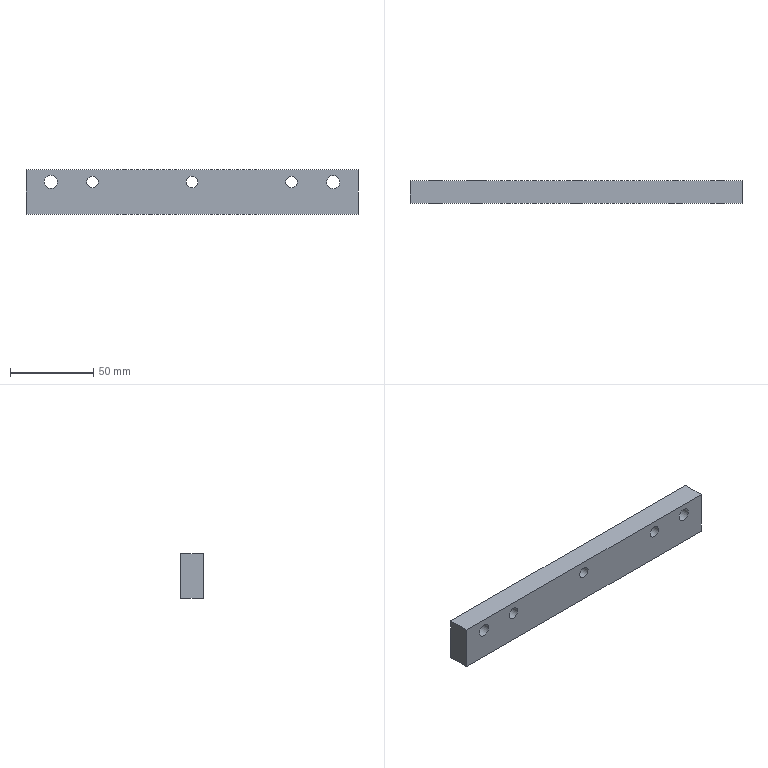Part | STEP file | SN10_002_006_GUIA | 1 solid | 17 faces | box 200 x 13.5 x 27 mm | volume 68797 mm3 | plane 9 | cylinder 8 | commonest cylinder face diameters 7 x3 11 x3 8 x2
STEP:
#1=CARTESIAN_POINT('',(0.,0.,0.));
#2=DIRECTION('',(0.,0.,1.));
#3=DIRECTION('',(1.,0.,0.));
#4=AXIS2_PLACEMENT_3D('',#1,#2,#3);
#5=CARTESIAN_POINT('',(88.51,228.5,59.418));
#6=VERTEX_POINT('',#5);
#7=CARTESIAN_POINT('',(85.,228.5,57.5));
#8=DIRECTION('',(0.,-1.,0.));
#9=DIRECTION('',(1.,0.,0.));
#10=AXIS2_PLACEMENT_3D('',#7,#8,#9);
#11=CIRCLE('',#10,4.);
#12=CARTESIAN_POINT('',(85.,228.4,57.5));
#13=DIRECTION('',(0.,-1.,0.));
#14=DIRECTION('',(0.8776,0.,0.4794));
#15=AXIS2_PLACEMENT_3D('',#12,#13,#14);
#16=CYLINDRICAL_SURFACE('',#15,4.);
#17=CARTESIAN_POINT('',(-0.5,-0.1));
#18=DIRECTION('',(1.,0.));
#19=VECTOR('',#18,1.);
#20=LINE('',#17,#19);
#21=(GEOMETRIC_REPRESENTATION_CONTEXT(2)PARAMETRIC_REPRESENTATION_CONTEXT()REPRESENTATION_CONTEXT('',''));
#22=DEFINITIONAL_REPRESENTATION('',(#20),#21);
#23=PCURVE('',#16,#22);
#24=CARTESIAN_POINT('',(0.,228.5,65.));
#25=DIRECTION('',(0.,-1.,0.));
#26=DIRECTION('',(0.,0.,-1.));
#27=AXIS2_PLACEMENT_3D('',#24,#25,#26);
#28=PLANE('',#27);
#29=CARTESIAN_POINT('',(7.5,85.));
#30=DIRECTION('',(0.,1.));
#31=AXIS2_PLACEMENT_2D('',#29,#30);
#32=CIRCLE('',#31,4.);
#33=(GEOMETRIC_REPRESENTATION_CONTEXT(2)PARAMETRIC_REPRESENTATION_CONTEXT()REPRESENTATION_CONTEXT('',''));
#34=DEFINITIONAL_REPRESENTATION('',(#32),#33);
#35=PCURVE('',#28,#34);
#36=SURFACE_CURVE('',#11,(#23,#35),.PCURVE_S1.);
#37=EDGE_CURVE('',#6,#6,#36,.T.);
#38=ORIENTED_EDGE('',*,*,#37,.T.);
#39=CARTESIAN_POINT('',(88.51,215.,59.418));
#40=VERTEX_POINT('',#39);
#41=CARTESIAN_POINT('',(88.51,228.5,59.418));
#42=CARTESIAN_POINT('',(88.51,215.,59.418));
#43=B_SPLINE_CURVE_WITH_KNOTS('',1,(#41,#42),.UNSPECIFIED.,.F.,.F.,(2,2),(-0.1,13.4),.PIECEWISE_BEZIER_KNOTS.);
#44=CARTESIAN_POINT('',(6.283,0.));
#45=DIRECTION('',(0.,1.));
#46=VECTOR('',#45,1.);
#47=LINE('',#44,#46);
#48=(GEOMETRIC_REPRESENTATION_CONTEXT(2)PARAMETRIC_REPRESENTATION_CONTEXT()REPRESENTATION_CONTEXT('',''));
#49=DEFINITIONAL_REPRESENTATION('',(#47),#48);
#50=PCURVE('',#16,#49);
#51=CARTESIAN_POINT('',(0.,0.));
#52=DIRECTION('',(0.,1.));
#53=VECTOR('',#52,1.);
#54=LINE('',#51,#53);
#55=(GEOMETRIC_REPRESENTATION_CONTEXT(2)PARAMETRIC_REPRESENTATION_CONTEXT()REPRESENTATION_CONTEXT('',''));
#56=DEFINITIONAL_REPRESENTATION('',(#54),#55);
#57=PCURVE('',#16,#56);
#58=SEAM_CURVE('',#43,(#50,#57),.PCURVE_S1.);
#59=EDGE_CURVE('',#6,#40,#58,.T.);
#60=ORIENTED_EDGE('',*,*,#59,.T.);
#61=CARTESIAN_POINT('',(85.,215.,57.5));
#62=DIRECTION('',(0.,-1.,0.));
#63=DIRECTION('',(1.,0.,0.));
#64=AXIS2_PLACEMENT_3D('',#61,#62,#63);
#65=CIRCLE('',#64,4.);
#66=CARTESIAN_POINT('',(-0.5,13.4));
#67=DIRECTION('',(1.,0.));
#68=VECTOR('',#67,1.);
#69=LINE('',#66,#68);
#70=(GEOMETRIC_REPRESENTATION_CONTEXT(2)PARAMETRIC_REPRESENTATION_CONTEXT()REPRESENTATION_CONTEXT('',''));
#71=DEFINITIONAL_REPRESENTATION('',(#69),#70);
#72=PCURVE('',#16,#71);
#73=CARTESIAN_POINT('',(0.,215.,38.));
#74=DIRECTION('',(0.,1.,0.));
#75=DIRECTION('',(0.,0.,1.));
#76=AXIS2_PLACEMENT_3D('',#73,#74,#75);
#77=PLANE('',#76);
#78=CARTESIAN_POINT('',(19.5,89.));
#79=CARTESIAN_POINT('',(26.428,89.));
#80=CARTESIAN_POINT('',(22.964,83.));
#81=CARTESIAN_POINT('',(19.5,77.));
#82=CARTESIAN_POINT('',(16.036,83.));
#83=CARTESIAN_POINT('',(12.572,89.));
#84=CARTESIAN_POINT('',(19.5,89.));
#85=(BOUNDED_CURVE()B_SPLINE_CURVE(2,(#78,#79,#80,#81,#82,#83,#84),.UNSPECIFIED.,.T.,.F.)B_SPLINE_CURVE_WITH_KNOTS((1,2,2,2,2,1),(-2.094,0.,2.094,4.189,6.283,8.378),.UNSPECIFIED.)CURVE()GEOMETRIC_REPRESENTATION_ITEM()RATIONAL_B_SPLINE_CURVE((1.,0.5,1.,0.5,1.,0.5,1.))REPRESENTATION_ITEM(''));
#86=(GEOMETRIC_REPRESENTATION_CONTEXT(2)PARAMETRIC_REPRESENTATION_CONTEXT()REPRESENTATION_CONTEXT('',''));
#87=DEFINITIONAL_REPRESENTATION('',(#85),#86);
#88=PCURVE('',#77,#87);
#89=SURFACE_CURVE('',#65,(#72,#88),.PCURVE_S1.);
#90=EDGE_CURVE('',#40,#40,#89,.T.);
#91=ORIENTED_EDGE('',*,*,#90,.F.);
#92=ORIENTED_EDGE('',*,*,#59,.F.);
#93=EDGE_LOOP('',(#38,#60,#91,#92));
#94=FACE_BOUND('',#93,.F.);
#95=ADVANCED_FACE('',(#94),#16,.F.);
#96=CARTESIAN_POINT('',(-100.,228.5,65.));
#97=VERTEX_POINT('',#96);
#98=CARTESIAN_POINT('',(100.,228.5,65.));
#99=VERTEX_POINT('',#98);
#100=CARTESIAN_POINT('',(-100.,228.5,65.));
#101=DIRECTION('',(1.,0.,0.));
#102=VECTOR('',#101,1.);
#103=LINE('',#100,#102);
#104=CARTESIAN_POINT('',(0.,215.,65.));
#105=DIRECTION('',(0.,0.,-1.));
#106=DIRECTION('',(-1.,0.,0.));
#107=AXIS2_PLACEMENT_3D('',#104,#105,#106);
#108=PLANE('',#107);
#109=CARTESIAN_POINT('',(100.,13.5));
#110=DIRECTION('',(-1.,0.));
#111=VECTOR('',#110,1.);
#112=LINE('',#109,#111);
#113=(GEOMETRIC_REPRESENTATION_CONTEXT(2)PARAMETRIC_REPRESENTATION_CONTEXT()REPRESENTATION_CONTEXT('',''));
#114=DEFINITIONAL_REPRESENTATION('',(#112),#113);
#115=PCURVE('',#108,#114);
#116=CARTESIAN_POINT('',(0.,-100.));
#117=DIRECTION('',(0.,1.));
#118=VECTOR('',#117,1.);
#119=LINE('',#116,#118);
#120=(GEOMETRIC_REPRESENTATION_CONTEXT(2)PARAMETRIC_REPRESENTATION_CONTEXT()REPRESENTATION_CONTEXT('',''));
#121=DEFINITIONAL_REPRESENTATION('',(#119),#120);
#122=PCURVE('',#28,#121);
#123=SURFACE_CURVE('',#103,(#115,#122),.PCURVE_S1.);
#124=EDGE_CURVE('',#97,#99,#123,.T.);
#125=ORIENTED_EDGE('',*,*,#124,.F.);
#126=CARTESIAN_POINT('',(-100.,215.,65.));
#127=VERTEX_POINT('',#126);
#128=CARTESIAN_POINT('',(-100.,215.,65.));
#129=DIRECTION('',(0.,1.,0.));
#130=VECTOR('',#129,1.);
#131=LINE('',#128,#130);
#132=CARTESIAN_POINT('',(100.,0.));
#133=DIRECTION('',(0.,1.));
#134=VECTOR('',#133,1.);
#135=LINE('',#132,#134);
#136=(GEOMETRIC_REPRESENTATION_CONTEXT(2)PARAMETRIC_REPRESENTATION_CONTEXT()REPRESENTATION_CONTEXT('',''));
#137=DEFINITIONAL_REPRESENTATION('',(#135),#136);
#138=PCURVE('',#108,#137);
#139=CARTESIAN_POINT('',(-100.,0.,0.));
#140=DIRECTION('',(1.,0.,0.));
#141=DIRECTION('',(0.,0.,-1.));
#142=AXIS2_PLACEMENT_3D('',#139,#140,#141);
#143=PLANE('',#142);
#144=CARTESIAN_POINT('',(-65.,215.));
#145=DIRECTION('',(0.,1.));
#146=VECTOR('',#145,1.);
#147=LINE('',#144,#146);
#148=(GEOMETRIC_REPRESENTATION_CONTEXT(2)PARAMETRIC_REPRESENTATION_CONTEXT()REPRESENTATION_CONTEXT('',''));
#149=DEFINITIONAL_REPRESENTATION('',(#147),#148);
#150=PCURVE('',#143,#149);
#151=SURFACE_CURVE('',#131,(#138,#150),.PCURVE_S1.);
#152=EDGE_CURVE('',#127,#97,#151,.T.);
#153=ORIENTED_EDGE('',*,*,#152,.F.);
#154=CARTESIAN_POINT('',(100.,215.,65.));
#155=VERTEX_POINT('',#154);
#156=CARTESIAN_POINT('',(-100.,215.,65.));
#157=DIRECTION('',(1.,0.,0.));
#158=VECTOR('',#157,1.);
#159=LINE('',#156,#158);
#160=CARTESIAN_POINT('',(100.,0.));
#161=DIRECTION('',(-1.,0.));
#162=VECTOR('',#161,1.);
#163=LINE('',#160,#162);
#164=(GEOMETRIC_REPRESENTATION_CONTEXT(2)PARAMETRIC_REPRESENTATION_CONTEXT()REPRESENTATION_CONTEXT('',''));
#165=DEFINITIONAL_REPRESENTATION('',(#163),#164);
#166=PCURVE('',#108,#165);
#167=CARTESIAN_POINT('',(27.,-100.));
#168=DIRECTION('',(0.,1.));
#169=VECTOR('',#168,1.);
#170=LINE('',#167,#169);
#171=(GEOMETRIC_REPRESENTATION_CONTEXT(2)PARAMETRIC_REPRESENTATION_CONTEXT()REPRESENTATION_CONTEXT('',''));
#172=DEFINITIONAL_REPRESENTATION('',(#170),#171);
#173=PCURVE('',#77,#172);
#174=SURFACE_CURVE('',#159,(#166,#173),.PCURVE_S1.);
#175=EDGE_CURVE('',#127,#155,#174,.T.);
#176=ORIENTED_EDGE('',*,*,#175,.T.);
#177=CARTESIAN_POINT('',(100.,215.,65.));
#178=DIRECTION('',(0.,1.,0.));
#179=VECTOR('',#178,1.);
#180=LINE('',#177,#179);
#181=CARTESIAN_POINT('',(-100.,0.));
#182=DIRECTION('',(0.,1.));
#183=VECTOR('',#182,1.);
#184=LINE('',#181,#183);
#185=(GEOMETRIC_REPRESENTATION_CONTEXT(2)PARAMETRIC_REPRESENTATION_CONTEXT()REPRESENTATION_CONTEXT('',''));
#186=DEFINITIONAL_REPRESENTATION('',(#184),#185);
#187=PCURVE('',#108,#186);
#188=CARTESIAN_POINT('',(100.,0.,0.));
#189=DIRECTION('',(1.,0.,0.));
#190=DIRECTION('',(0.,0.,-1.));
#191=AXIS2_PLACEMENT_3D('',#188,#189,#190);
#192=PLANE('',#191);
#193=CARTESIAN_POINT('',(-65.,215.));
#194=DIRECTION('',(0.,1.));
#195=VECTOR('',#194,1.);
#196=LINE('',#193,#195);
#197=(GEOMETRIC_REPRESENTATION_CONTEXT(2)PARAMETRIC_REPRESENTATION_CONTEXT()REPRESENTATION_CONTEXT('',''));
#198=DEFINITIONAL_REPRESENTATION('',(#196),#197);
#199=PCURVE('',#192,#198);
#200=SURFACE_CURVE('',#180,(#187,#199),.PCURVE_S1.);
#201=EDGE_CURVE('',#155,#99,#200,.T.);
#202=ORIENTED_EDGE('',*,*,#201,.T.);
#203=EDGE_LOOP('',(#125,#153,#176,#202));
#204=FACE_BOUND('',#203,.T.);
#205=ADVANCED_FACE('',(#204),#108,.F.);
#206=CARTESIAN_POINT('',(-100.,228.5,38.));
#207=VERTEX_POINT('',#206);
#208=CARTESIAN_POINT('',(-100.,228.5,65.));
#209=DIRECTION('',(0.,0.,-1.));
#210=VECTOR('',#209,1.);
#211=LINE('',#208,#210);
#212=CARTESIAN_POINT('',(-65.,228.5));
#213=DIRECTION('',(1.,0.));
#214=VECTOR('',#213,1.);
#215=LINE('',#212,#214);
#216=(GEOMETRIC_REPRESENTATION_CONTEXT(2)PARAMETRIC_REPRESENTATION_CONTEXT()REPRESENTATION_CONTEXT('',''));
#217=DEFINITIONAL_REPRESENTATION('',(#215),#216);
#218=PCURVE('',#143,#217);
#219=CARTESIAN_POINT('',(0.,-100.));
#220=DIRECTION('',(1.,0.));
#221=VECTOR('',#220,1.);
#222=LINE('',#219,#221);
#223=(GEOMETRIC_REPRESENTATION_CONTEXT(2)PARAMETRIC_REPRESENTATION_CONTEXT()REPRESENTATION_CONTEXT('',''));
#224=DEFINITIONAL_REPRESENTATION('',(#222),#223);
#225=PCURVE('',#28,#224);
#226=SURFACE_CURVE('',#211,(#218,#225),.PCURVE_S1.);
#227=EDGE_CURVE('',#97,#207,#226,.T.);
#228=ORIENTED_EDGE('',*,*,#227,.T.);
#229=CARTESIAN_POINT('',(-100.,215.,38.));
#230=VERTEX_POINT('',#229);
#231=CARTESIAN_POINT('',(-100.,228.5,38.));
#232=DIRECTION('',(0.,-1.,0.));
#233=VECTOR('',#232,1.);
#234=LINE('',#231,#233);
#235=CARTESIAN_POINT('',(-38.,228.5));
#236=DIRECTION('',(0.,-1.));
#237=VECTOR('',#236,1.);
#238=LINE('',#235,#237);
#239=(GEOMETRIC_REPRESENTATION_CONTEXT(2)PARAMETRIC_REPRESENTATION_CONTEXT()REPRESENTATION_CONTEXT('',''));
#240=DEFINITIONAL_REPRESENTATION('',(#238),#239);
#241=PCURVE('',#143,#240);
#242=CARTESIAN_POINT('',(0.,228.5,38.));
#243=DIRECTION('',(0.,0.,1.));
#244=DIRECTION('',(1.,0.,0.));
#245=AXIS2_PLACEMENT_3D('',#242,#243,#244);
#246=PLANE('',#245);
#247=CARTESIAN_POINT('',(-100.,0.));
#248=DIRECTION('',(0.,-1.));
#249=VECTOR('',#248,1.);
#250=LINE('',#247,#249);
#251=(GEOMETRIC_REPRESENTATION_CONTEXT(2)PARAMETRIC_REPRESENTATION_CONTEXT()REPRESENTATION_CONTEXT('',''));
#252=DEFINITIONAL_REPRESENTATION('',(#250),#251);
#253=PCURVE('',#246,#252);
#254=SURFACE_CURVE('',#234,(#241,#253),.PCURVE_S1.);
#255=EDGE_CURVE('',#207,#230,#254,.T.);
#256=ORIENTED_EDGE('',*,*,#255,.T.);
#257=CARTESIAN_POINT('',(-100.,215.,38.));
#258=DIRECTION('',(0.,0.,1.));
#259=VECTOR('',#258,1.);
#260=LINE('',#257,#259);
#261=CARTESIAN_POINT('',(-38.,215.));
#262=DIRECTION('',(-1.,0.));
#263=VECTOR('',#262,1.);
#264=LINE('',#261,#263);
#265=(GEOMETRIC_REPRESENTATION_CONTEXT(2)PARAMETRIC_REPRESENTATION_CONTEXT()REPRESENTATION_CONTEXT('',''));
#266=DEFINITIONAL_REPRESENTATION('',(#264),#265);
#267=PCURVE('',#143,#266);
#268=CARTESIAN_POINT('',(0.,-100.));
#269=DIRECTION('',(1.,0.));
#270=VECTOR('',#269,1.);
#271=LINE('',#268,#270);
#272=(GEOMETRIC_REPRESENTATION_CONTEXT(2)PARAMETRIC_REPRESENTATION_CONTEXT()REPRESENTATION_CONTEXT('',''));
#273=DEFINITIONAL_REPRESENTATION('',(#271),#272);
#274=PCURVE('',#77,#273);
#275=SURFACE_CURVE('',#260,(#267,#274),.PCURVE_S1.);
#276=EDGE_CURVE('',#230,#127,#275,.T.);
#277=ORIENTED_EDGE('',*,*,#276,.T.);
#278=ORIENTED_EDGE('',*,*,#152,.T.);
#279=EDGE_LOOP('',(#228,#256,#277,#278));
#280=FACE_BOUND('',#279,.T.);
#281=ADVANCED_FACE('',(#280),#143,.F.);
#282=CARTESIAN_POINT('',(55.173,228.5,54.863));
#283=VERTEX_POINT('',#282);
#284=CARTESIAN_POINT('',(60.,228.5,57.5));
#285=DIRECTION('',(0.,-1.,0.));
#286=DIRECTION('',(1.,0.,0.));
#287=AXIS2_PLACEMENT_3D('',#284,#285,#286);
#288=CIRCLE('',#287,5.5);
#289=CARTESIAN_POINT('',(60.,228.4,57.5));
#290=DIRECTION('',(0.,-1.,0.));
#291=DIRECTION('',(0.8776,0.,0.4794));
#292=AXIS2_PLACEMENT_3D('',#289,#290,#291);
#293=CYLINDRICAL_SURFACE('',#292,5.5);
#294=CARTESIAN_POINT('',(-0.5,-0.1));
#295=DIRECTION('',(1.,0.));
#296=VECTOR('',#295,1.);
#297=LINE('',#294,#296);
#298=(GEOMETRIC_REPRESENTATION_CONTEXT(2)PARAMETRIC_REPRESENTATION_CONTEXT()REPRESENTATION_CONTEXT('',''));
#299=DEFINITIONAL_REPRESENTATION('',(#297),#298);
#300=PCURVE('',#293,#299);
#301=CARTESIAN_POINT('',(7.5,60.));
#302=DIRECTION('',(0.,1.));
#303=AXIS2_PLACEMENT_2D('',#301,#302);
#304=CIRCLE('',#303,5.5);
#305=(GEOMETRIC_REPRESENTATION_CONTEXT(2)PARAMETRIC_REPRESENTATION_CONTEXT()REPRESENTATION_CONTEXT('',''));
#306=DEFINITIONAL_REPRESENTATION('',(#304),#305);
#307=PCURVE('',#28,#306);
#308=SURFACE_CURVE('',#288,(#300,#307),.PCURVE_S1.);
#309=EDGE_CURVE('',#283,#283,#308,.T.);
#310=ORIENTED_EDGE('',*,*,#309,.T.);
#311=CARTESIAN_POINT('',(55.173,221.5,54.863));
#312=VERTEX_POINT('',#311);
#313=CARTESIAN_POINT('',(55.173,228.5,54.863));
#314=CARTESIAN_POINT('',(55.173,221.5,54.863));
#315=B_SPLINE_CURVE_WITH_KNOTS('',1,(#313,#314),.UNSPECIFIED.,.F.,.F.,(2,2),(-0.1,6.9),.PIECEWISE_BEZIER_KNOTS.);
#316=CARTESIAN_POINT('',(9.425,0.));
#317=DIRECTION('',(0.,1.));
#318=VECTOR('',#317,1.);
#319=LINE('',#316,#318);
#320=(GEOMETRIC_REPRESENTATION_CONTEXT(2)PARAMETRIC_REPRESENTATION_CONTEXT()REPRESENTATION_CONTEXT('',''));
#321=DEFINITIONAL_REPRESENTATION('',(#319),#320);
#322=PCURVE('',#293,#321);
#323=CARTESIAN_POINT('',(3.142,0.));
#324=DIRECTION('',(0.,1.));
#325=VECTOR('',#324,1.);
#326=LINE('',#323,#325);
#327=(GEOMETRIC_REPRESENTATION_CONTEXT(2)PARAMETRIC_REPRESENTATION_CONTEXT()REPRESENTATION_CONTEXT('',''));
#328=DEFINITIONAL_REPRESENTATION('',(#326),#327);
#329=PCURVE('',#293,#328);
#330=SEAM_CURVE('',#315,(#322,#329),.PCURVE_S1.);
#331=EDGE_CURVE('',#283,#312,#330,.T.);
#332=ORIENTED_EDGE('',*,*,#331,.T.);
#333=CARTESIAN_POINT('',(60.,221.5,57.5));
#334=DIRECTION('',(0.,-1.,0.));
#335=DIRECTION('',(1.,0.,0.));
#336=AXIS2_PLACEMENT_3D('',#333,#334,#335);
#337=CIRCLE('',#336,5.5);
#338=CARTESIAN_POINT('',(-0.5,6.9));
#339=DIRECTION('',(1.,0.));
#340=VECTOR('',#339,1.);
#341=LINE('',#338,#340);
#342=(GEOMETRIC_REPRESENTATION_CONTEXT(2)PARAMETRIC_REPRESENTATION_CONTEXT()REPRESENTATION_CONTEXT('',''));
#343=DEFINITIONAL_REPRESENTATION('',(#341),#342);
#344=PCURVE('',#293,#343);
#345=CARTESIAN_POINT('',(63.5,221.5,57.5));
#346=DIRECTION('',(0.,-1.,0.));
#347=DIRECTION('',(0.,0.,-1.));
#348=AXIS2_PLACEMENT_3D('',#345,#346,#347);
#349=PLANE('',#348);
#350=CARTESIAN_POINT('',(0.,-3.5));
#351=DIRECTION('',(0.,1.));
#352=AXIS2_PLACEMENT_2D('',#350,#351);
#353=CIRCLE('',#352,5.5);
#354=(GEOMETRIC_REPRESENTATION_CONTEXT(2)PARAMETRIC_REPRESENTATION_CONTEXT()REPRESENTATION_CONTEXT('',''));
#355=DEFINITIONAL_REPRESENTATION('',(#353),#354);
#356=PCURVE('',#349,#355);
#357=SURFACE_CURVE('',#337,(#344,#356),.PCURVE_S1.);
#358=EDGE_CURVE('',#312,#312,#357,.T.);
#359=ORIENTED_EDGE('',*,*,#358,.F.);
#360=ORIENTED_EDGE('',*,*,#331,.F.);
#361=EDGE_LOOP('',(#310,#332,#359,#360));
#362=FACE_BOUND('',#361,.F.);
#363=ADVANCED_FACE('',(#362),#293,.F.);
#364=CARTESIAN_POINT('',(-4.827,228.5,54.863));
#365=VERTEX_POINT('',#364);
#366=CARTESIAN_POINT('',(0.,228.5,57.5));
#367=DIRECTION('',(0.,-1.,0.));
#368=DIRECTION('',(1.,0.,0.));
#369=AXIS2_PLACEMENT_3D('',#366,#367,#368);
#370=CIRCLE('',#369,5.5);
#371=CARTESIAN_POINT('',(0.,228.4,57.5));
#372=DIRECTION('',(0.,-1.,0.));
#373=DIRECTION('',(0.8776,0.,0.4794));
#374=AXIS2_PLACEMENT_3D('',#371,#372,#373);
#375=CYLINDRICAL_SURFACE('',#374,5.5);
#376=CARTESIAN_POINT('',(-0.5,-0.1));
#377=DIRECTION('',(1.,0.));
#378=VECTOR('',#377,1.);
#379=LINE('',#376,#378);
#380=(GEOMETRIC_REPRESENTATION_CONTEXT(2)PARAMETRIC_REPRESENTATION_CONTEXT()REPRESENTATION_CONTEXT('',''));
#381=DEFINITIONAL_REPRESENTATION('',(#379),#380);
#382=PCURVE('',#375,#381);
#383=CARTESIAN_POINT('',(7.5,0.));
#384=DIRECTION('',(0.,1.));
#385=AXIS2_PLACEMENT_2D('',#383,#384);
#386=CIRCLE('',#385,5.5);
#387=(GEOMETRIC_REPRESENTATION_CONTEXT(2)PARAMETRIC_REPRESENTATION_CONTEXT()REPRESENTATION_CONTEXT('',''));
#388=DEFINITIONAL_REPRESENTATION('',(#386),#387);
#389=PCURVE('',#28,#388);
#390=SURFACE_CURVE('',#370,(#382,#389),.PCURVE_S1.);
#391=EDGE_CURVE('',#365,#365,#390,.T.);
#392=ORIENTED_EDGE('',*,*,#391,.T.);
#393=CARTESIAN_POINT('',(-4.827,221.5,54.863));
#394=VERTEX_POINT('',#393);
#395=CARTESIAN_POINT('',(-4.827,228.5,54.863));
#396=CARTESIAN_POINT('',(-4.827,221.5,54.863));
#397=B_SPLINE_CURVE_WITH_KNOTS('',1,(#395,#396),.UNSPECIFIED.,.F.,.F.,(2,2),(-0.1,6.9),.PIECEWISE_BEZIER_KNOTS.);
#398=CARTESIAN_POINT('',(9.425,0.));
#399=DIRECTION('',(0.,1.));
#400=VECTOR('',#399,1.);
#401=LINE('',#398,#400);
#402=(GEOMETRIC_REPRESENTATION_CONTEXT(2)PARAMETRIC_REPRESENTATION_CONTEXT()REPRESENTATION_CONTEXT('',''));
#403=DEFINITIONAL_REPRESENTATION('',(#401),#402);
#404=PCURVE('',#375,#403);
#405=CARTESIAN_POINT('',(3.142,0.));
#406=DIRECTION('',(0.,1.));
#407=VECTOR('',#406,1.);
#408=LINE('',#405,#407);
#409=(GEOMETRIC_REPRESENTATION_CONTEXT(2)PARAMETRIC_REPRESENTATION_CONTEXT()REPRESENTATION_CONTEXT('',''));
#410=DEFINITIONAL_REPRESENTATION('',(#408),#409);
#411=PCURVE('',#375,#410);
#412=SEAM_CURVE('',#397,(#404,#411),.PCURVE_S1.);
#413=EDGE_CURVE('',#365,#394,#412,.T.);
#414=ORIENTED_EDGE('',*,*,#413,.T.);
#415=CARTESIAN_POINT('',(0.,221.5,57.5));
#416=DIRECTION('',(0.,-1.,0.));
#417=DIRECTION('',(1.,0.,0.));
#418=AXIS2_PLACEMENT_3D('',#415,#416,#417);
#419=CIRCLE('',#418,5.5);
#420=CARTESIAN_POINT('',(-0.5,6.9));
#421=DIRECTION('',(1.,0.));
#422=VECTOR('',#421,1.);
#423=LINE('',#420,#422);
#424=(GEOMETRIC_REPRESENTATION_CONTEXT(2)PARAMETRIC_REPRESENTATION_CONTEXT()REPRESENTATION_CONTEXT('',''));
#425=DEFINITIONAL_REPRESENTATION('',(#423),#424);
#426=PCURVE('',#375,#425);
#427=CARTESIAN_POINT('',(63.5,221.5,57.5));
#428=DIRECTION('',(0.,-1.,0.));
#429=DIRECTION('',(0.,0.,-1.));
#430=AXIS2_PLACEMENT_3D('',#427,#428,#429);
#431=PLANE('',#430);
#432=CARTESIAN_POINT('',(0.,-63.5));
#433=DIRECTION('',(0.,1.));
#434=AXIS2_PLACEMENT_2D('',#432,#433);
#435=CIRCLE('',#434,5.5);
#436=(GEOMETRIC_REPRESENTATION_CONTEXT(2)PARAMETRIC_REPRESENTATION_CONTEXT()REPRESENTATION_CONTEXT('',''));
#437=DEFINITIONAL_REPRESENTATION('',(#435),#436);
#438=PCURVE('',#431,#437);
#439=SURFACE_CURVE('',#419,(#426,#438),.PCURVE_S1.);
#440=EDGE_CURVE('',#394,#394,#439,.T.);
#441=ORIENTED_EDGE('',*,*,#440,.F.);
#442=ORIENTED_EDGE('',*,*,#413,.F.);
#443=EDGE_LOOP('',(#392,#414,#441,#442));
#444=FACE_BOUND('',#443,.F.);
#445=ADVANCED_FACE('',(#444),#375,.F.);
#446=CARTESIAN_POINT('',(-64.827,228.5,54.863));
#447=VERTEX_POINT('',#446);
#448=CARTESIAN_POINT('',(-60.,228.5,57.5));
#449=DIRECTION('',(0.,-1.,0.));
#450=DIRECTION('',(1.,0.,0.));
#451=AXIS2_PLACEMENT_3D('',#448,#449,#450);
#452=CIRCLE('',#451,5.5);
#453=CARTESIAN_POINT('',(-60.,228.4,57.5));
#454=DIRECTION('',(0.,-1.,0.));
#455=DIRECTION('',(0.8776,0.,0.4794));
#456=AXIS2_PLACEMENT_3D('',#453,#454,#455);
#457=CYLINDRICAL_SURFACE('',#456,5.5);
#458=CARTESIAN_POINT('',(-0.5,-0.1));
#459=DIRECTION('',(1.,0.));
#460=VECTOR('',#459,1.);
#461=LINE('',#458,#460);
#462=(GEOMETRIC_REPRESENTATION_CONTEXT(2)PARAMETRIC_REPRESENTATION_CONTEXT()REPRESENTATION_CONTEXT('',''));
#463=DEFINITIONAL_REPRESENTATION('',(#461),#462);
#464=PCURVE('',#457,#463);
#465=CARTESIAN_POINT('',(7.5,-60.));
#466=DIRECTION('',(0.,1.));
#467=AXIS2_PLACEMENT_2D('',#465,#466);
#468=CIRCLE('',#467,5.5);
#469=(GEOMETRIC_REPRESENTATION_CONTEXT(2)PARAMETRIC_REPRESENTATION_CONTEXT()REPRESENTATION_CONTEXT('',''));
#470=DEFINITIONAL_REPRESENTATION('',(#468),#469);
#471=PCURVE('',#28,#470);
#472=SURFACE_CURVE('',#452,(#464,#471),.PCURVE_S1.);
#473=EDGE_CURVE('',#447,#447,#472,.T.);
#474=ORIENTED_EDGE('',*,*,#473,.T.);
#475=CARTESIAN_POINT('',(-64.827,221.5,54.863));
#476=VERTEX_POINT('',#475);
#477=CARTESIAN_POINT('',(-64.827,228.5,54.863));
#478=CARTESIAN_POINT('',(-64.827,221.5,54.863));
#479=B_SPLINE_CURVE_WITH_KNOTS('',1,(#477,#478),.UNSPECIFIED.,.F.,.F.,(2,2),(-0.1,6.9),.PIECEWISE_BEZIER_KNOTS.);
#480=CARTESIAN_POINT('',(9.425,0.));
#481=DIRECTION('',(0.,1.));
#482=VECTOR('',#481,1.);
#483=LINE('',#480,#482);
#484=(GEOMETRIC_REPRESENTATION_CONTEXT(2)PARAMETRIC_REPRESENTATION_CONTEXT()REPRESENTATION_CONTEXT('',''));
#485=DEFINITIONAL_REPRESENTATION('',(#483),#484);
#486=PCURVE('',#457,#485);
#487=CARTESIAN_POINT('',(3.142,0.));
#488=DIRECTION('',(0.,1.));
#489=VECTOR('',#488,1.);
#490=LINE('',#487,#489);
#491=(GEOMETRIC_REPRESENTATION_CONTEXT(2)PARAMETRIC_REPRESENTATION_CONTEXT()REPRESENTATION_CONTEXT('',''));
#492=DEFINITIONAL_REPRESENTATION('',(#490),#491);
#493=PCURVE('',#457,#492);
#494=SEAM_CURVE('',#479,(#486,#493),.PCURVE_S1.);
#495=EDGE_CURVE('',#447,#476,#494,.T.);
#496=ORIENTED_EDGE('',*,*,#495,.T.);
#497=CARTESIAN_POINT('',(-60.,221.5,57.5));
#498=DIRECTION('',(0.,-1.,0.));
#499=DIRECTION('',(1.,0.,0.));
#500=AXIS2_PLACEMENT_3D('',#497,#498,#499);
#501=CIRCLE('',#500,5.5);
#502=CARTESIAN_POINT('',(-0.5,6.9));
#503=DIRECTION('',(1.,0.));
#504=VECTOR('',#503,1.);
#505=LINE('',#502,#504);
#506=(GEOMETRIC_REPRESENTATION_CONTEXT(2)PARAMETRIC_REPRESENTATION_CONTEXT()REPRESENTATION_CONTEXT('',''));
#507=DEFINITIONAL_REPRESENTATION('',(#505),#506);
#508=PCURVE('',#457,#507);
#509=CARTESIAN_POINT('',(63.5,221.5,57.5));
#510=DIRECTION('',(0.,-1.,0.));
#511=DIRECTION('',(0.,0.,-1.));
#512=AXIS2_PLACEMENT_3D('',#509,#510,#511);
#513=PLANE('',#512);
#514=CARTESIAN_POINT('',(0.,-123.5));
#515=DIRECTION('',(0.,1.));
#516=AXIS2_PLACEMENT_2D('',#514,#515);
#517=CIRCLE('',#516,5.5);
#518=(GEOMETRIC_REPRESENTATION_CONTEXT(2)PARAMETRIC_REPRESENTATION_CONTEXT()REPRESENTATION_CONTEXT('',''));
#519=DEFINITIONAL_REPRESENTATION('',(#517),#518);
#520=PCURVE('',#513,#519);
#521=SURFACE_CURVE('',#501,(#508,#520),.PCURVE_S1.);
#522=EDGE_CURVE('',#476,#476,#521,.T.);
#523=ORIENTED_EDGE('',*,*,#522,.F.);
#524=ORIENTED_EDGE('',*,*,#495,.F.);
#525=EDGE_LOOP('',(#474,#496,#523,#524));
#526=FACE_BOUND('',#525,.F.);
#527=ADVANCED_FACE('',(#526),#457,.F.);
#528=ORIENTED_EDGE('',*,*,#358,.F.);
#529=EDGE_LOOP('',(#528));
#530=FACE_BOUND('',#529,.T.);
#531=CARTESIAN_POINT('',(63.072,221.5,59.178));
#532=VERTEX_POINT('',#531);
#533=CARTESIAN_POINT('',(60.,221.5,57.5));
#534=DIRECTION('',(0.,-1.,0.));
#535=DIRECTION('',(1.,0.,0.));
#536=AXIS2_PLACEMENT_3D('',#533,#534,#535);
#537=CIRCLE('',#536,3.5);
#538=CARTESIAN_POINT('',(0.,-3.5));
#539=DIRECTION('',(0.,1.));
#540=AXIS2_PLACEMENT_2D('',#538,#539);
#541=CIRCLE('',#540,3.5);
#542=(GEOMETRIC_REPRESENTATION_CONTEXT(2)PARAMETRIC_REPRESENTATION_CONTEXT()REPRESENTATION_CONTEXT('',''));
#543=DEFINITIONAL_REPRESENTATION('',(#541),#542);
#544=PCURVE('',#349,#543);
#545=CARTESIAN_POINT('',(60.,228.4,57.5));
#546=DIRECTION('',(0.,-1.,0.));
#547=DIRECTION('',(0.8776,0.,0.4794));
#548=AXIS2_PLACEMENT_3D('',#545,#546,#547);
#549=CYLINDRICAL_SURFACE('',#548,3.5);
#550=CARTESIAN_POINT('',(-0.5,6.9));
#551=DIRECTION('',(1.,0.));
#552=VECTOR('',#551,1.);
#553=LINE('',#550,#552);
#554=(GEOMETRIC_REPRESENTATION_CONTEXT(2)PARAMETRIC_REPRESENTATION_CONTEXT()REPRESENTATION_CONTEXT('',''));
#555=DEFINITIONAL_REPRESENTATION('',(#553),#554);
#556=PCURVE('',#549,#555);
#557=SURFACE_CURVE('',#537,(#544,#556),.PCURVE_S1.);
#558=EDGE_CURVE('',#532,#532,#557,.T.);
#559=ORIENTED_EDGE('',*,*,#558,.T.);
#560=EDGE_LOOP('',(#559));
#561=FACE_BOUND('',#560,.T.);
#562=ADVANCED_FACE('',(#530,#561),#349,.F.);
#563=ORIENTED_EDGE('',*,*,#440,.F.);
#564=EDGE_LOOP('',(#563));
#565=FACE_BOUND('',#564,.T.);
#566=CARTESIAN_POINT('',(3.072,221.5,59.178));
#567=VERTEX_POINT('',#566);
#568=CARTESIAN_POINT('',(0.,221.5,57.5));
#569=DIRECTION('',(0.,-1.,0.));
#570=DIRECTION('',(1.,0.,0.));
#571=AXIS2_PLACEMENT_3D('',#568,#569,#570);
#572=CIRCLE('',#571,3.5);
#573=CARTESIAN_POINT('',(0.,-63.5));
#574=DIRECTION('',(0.,1.));
#575=AXIS2_PLACEMENT_2D('',#573,#574);
#576=CIRCLE('',#575,3.5);
#577=(GEOMETRIC_REPRESENTATION_CONTEXT(2)PARAMETRIC_REPRESENTATION_CONTEXT()REPRESENTATION_CONTEXT('',''));
#578=DEFINITIONAL_REPRESENTATION('',(#576),#577);
#579=PCURVE('',#431,#578);
#580=CARTESIAN_POINT('',(0.,228.4,57.5));
#581=DIRECTION('',(0.,-1.,0.));
#582=DIRECTION('',(0.8776,0.,0.4794));
#583=AXIS2_PLACEMENT_3D('',#580,#581,#582);
#584=CYLINDRICAL_SURFACE('',#583,3.5);
#585=CARTESIAN_POINT('',(-0.5,6.9));
#586=DIRECTION('',(1.,0.));
#587=VECTOR('',#586,1.);
#588=LINE('',#585,#587);
#589=(GEOMETRIC_REPRESENTATION_CONTEXT(2)PARAMETRIC_REPRESENTATION_CONTEXT()REPRESENTATION_CONTEXT('',''));
#590=DEFINITIONAL_REPRESENTATION('',(#588),#589);
#591=PCURVE('',#584,#590);
#592=SURFACE_CURVE('',#572,(#579,#591),.PCURVE_S1.);
#593=EDGE_CURVE('',#567,#567,#592,.T.);
#594=ORIENTED_EDGE('',*,*,#593,.T.);
#595=EDGE_LOOP('',(#594));
#596=FACE_BOUND('',#595,.T.);
#597=ADVANCED_FACE('',(#565,#596),#431,.F.);
#598=ORIENTED_EDGE('',*,*,#522,.F.);
#599=EDGE_LOOP('',(#598));
#600=FACE_BOUND('',#599,.T.);
#601=CARTESIAN_POINT('',(-56.928,221.5,59.178));
#602=VERTEX_POINT('',#601);
#603=CARTESIAN_POINT('',(-60.,221.5,57.5));
#604=DIRECTION('',(0.,-1.,0.));
#605=DIRECTION('',(1.,0.,0.));
#606=AXIS2_PLACEMENT_3D('',#603,#604,#605);
#607=CIRCLE('',#606,3.5);
#608=CARTESIAN_POINT('',(0.,-123.5));
#609=DIRECTION('',(0.,1.));
#610=AXIS2_PLACEMENT_2D('',#608,#609);
#611=CIRCLE('',#610,3.5);
#612=(GEOMETRIC_REPRESENTATION_CONTEXT(2)PARAMETRIC_REPRESENTATION_CONTEXT()REPRESENTATION_CONTEXT('',''));
#613=DEFINITIONAL_REPRESENTATION('',(#611),#612);
#614=PCURVE('',#513,#613);
#615=CARTESIAN_POINT('',(-60.,228.4,57.5));
#616=DIRECTION('',(0.,-1.,0.));
#617=DIRECTION('',(0.8776,0.,0.4794));
#618=AXIS2_PLACEMENT_3D('',#615,#616,#617);
#619=CYLINDRICAL_SURFACE('',#618,3.5);
#620=CARTESIAN_POINT('',(-0.5,6.9));
#621=DIRECTION('',(1.,0.));
#622=VECTOR('',#621,1.);
#623=LINE('',#620,#622);
#624=(GEOMETRIC_REPRESENTATION_CONTEXT(2)PARAMETRIC_REPRESENTATION_CONTEXT()REPRESENTATION_CONTEXT('',''));
#625=DEFINITIONAL_REPRESENTATION('',(#623),#624);
#626=PCURVE('',#619,#625);
#627=SURFACE_CURVE('',#607,(#614,#626),.PCURVE_S1.);
#628=EDGE_CURVE('',#602,#602,#627,.T.);
#629=ORIENTED_EDGE('',*,*,#628,.T.);
#630=EDGE_LOOP('',(#629));
#631=FACE_BOUND('',#630,.T.);
#632=ADVANCED_FACE('',(#600,#631),#513,.F.);
#633=CARTESIAN_POINT('',(63.072,215.,59.178));
#634=VERTEX_POINT('',#633);
#635=CARTESIAN_POINT('',(60.,215.,57.5));
#636=DIRECTION('',(0.,-1.,0.));
#637=DIRECTION('',(1.,0.,0.));
#638=AXIS2_PLACEMENT_3D('',#635,#636,#637);
#639=CIRCLE('',#638,3.5);
#640=CARTESIAN_POINT('',(-0.5,13.4));
#641=DIRECTION('',(1.,0.));
#642=VECTOR('',#641,1.);
#643=LINE('',#640,#642);
#644=(GEOMETRIC_REPRESENTATION_CONTEXT(2)PARAMETRIC_REPRESENTATION_CONTEXT()REPRESENTATION_CONTEXT('',''));
#645=DEFINITIONAL_REPRESENTATION('',(#643),#644);
#646=PCURVE('',#549,#645);
#647=CARTESIAN_POINT('',(19.5,63.5));
#648=CARTESIAN_POINT('',(25.562,63.5));
#649=CARTESIAN_POINT('',(22.531,58.25));
#650=CARTESIAN_POINT('',(19.5,53.));
#651=CARTESIAN_POINT('',(16.469,58.25));
#652=CARTESIAN_POINT('',(13.438,63.5));
#653=CARTESIAN_POINT('',(19.5,63.5));
#654=(BOUNDED_CURVE()B_SPLINE_CURVE(2,(#647,#648,#649,#650,#651,#652,#653),.UNSPECIFIED.,.T.,.F.)B_SPLINE_CURVE_WITH_KNOTS((1,2,2,2,2,1),(-2.094,0.,2.094,4.189,6.283,8.378),.UNSPECIFIED.)CURVE()GEOMETRIC_REPRESENTATION_ITEM()RATIONAL_B_SPLINE_CURVE((1.,0.5,1.,0.5,1.,0.5,1.))REPRESENTATION_ITEM(''));
#655=(GEOMETRIC_REPRESENTATION_CONTEXT(2)PARAMETRIC_REPRESENTATION_CONTEXT()REPRESENTATION_CONTEXT('',''));
#656=DEFINITIONAL_REPRESENTATION('',(#654),#655);
#657=PCURVE('',#77,#656);
#658=SURFACE_CURVE('',#639,(#646,#657),.PCURVE_S1.);
#659=EDGE_CURVE('',#634,#634,#658,.T.);
#660=ORIENTED_EDGE('',*,*,#659,.F.);
#661=CARTESIAN_POINT('',(63.072,221.5,59.178));
#662=CARTESIAN_POINT('',(63.072,215.,59.178));
#663=B_SPLINE_CURVE_WITH_KNOTS('',1,(#661,#662),.UNSPECIFIED.,.F.,.F.,(2,2),(6.9,13.4),.PIECEWISE_BEZIER_KNOTS.);
#664=CARTESIAN_POINT('',(0.,0.));
#665=DIRECTION('',(0.,1.));
#666=VECTOR('',#665,1.);
#667=LINE('',#664,#666);
#668=(GEOMETRIC_REPRESENTATION_CONTEXT(2)PARAMETRIC_REPRESENTATION_CONTEXT()REPRESENTATION_CONTEXT('',''));
#669=DEFINITIONAL_REPRESENTATION('',(#667),#668);
#670=PCURVE('',#549,#669);
#671=CARTESIAN_POINT('',(6.283,0.));
#672=DIRECTION('',(0.,1.));
#673=VECTOR('',#672,1.);
#674=LINE('',#671,#673);
#675=(GEOMETRIC_REPRESENTATION_CONTEXT(2)PARAMETRIC_REPRESENTATION_CONTEXT()REPRESENTATION_CONTEXT('',''));
#676=DEFINITIONAL_REPRESENTATION('',(#674),#675);
#677=PCURVE('',#549,#676);
#678=SEAM_CURVE('',#663,(#670,#677),.PCURVE_S1.);
#679=EDGE_CURVE('',#532,#634,#678,.T.);
#680=ORIENTED_EDGE('',*,*,#679,.F.);
#681=ORIENTED_EDGE('',*,*,#558,.T.);
#682=ORIENTED_EDGE('',*,*,#679,.T.);
#683=EDGE_LOOP('',(#660,#680,#681,#682));
#684=FACE_BOUND('',#683,.F.);
#685=ADVANCED_FACE('',(#684),#549,.F.);
#686=CARTESIAN_POINT('',(3.072,215.,59.178));
#687=VERTEX_POINT('',#686);
#688=CARTESIAN_POINT('',(0.,215.,57.5));
#689=DIRECTION('',(0.,-1.,0.));
#690=DIRECTION('',(1.,0.,0.));
#691=AXIS2_PLACEMENT_3D('',#688,#689,#690);
#692=CIRCLE('',#691,3.5);
#693=CARTESIAN_POINT('',(-0.5,13.4));
#694=DIRECTION('',(1.,0.));
#695=VECTOR('',#694,1.);
#696=LINE('',#693,#695);
#697=(GEOMETRIC_REPRESENTATION_CONTEXT(2)PARAMETRIC_REPRESENTATION_CONTEXT()REPRESENTATION_CONTEXT('',''));
#698=DEFINITIONAL_REPRESENTATION('',(#696),#697);
#699=PCURVE('',#584,#698);
#700=CARTESIAN_POINT('',(19.5,3.5));
#701=CARTESIAN_POINT('',(25.562,3.5));
#702=CARTESIAN_POINT('',(22.531,-1.75));
#703=CARTESIAN_POINT('',(19.5,-7.));
#704=CARTESIAN_POINT('',(16.469,-1.75));
#705=CARTESIAN_POINT('',(13.438,3.5));
#706=CARTESIAN_POINT('',(19.5,3.5));
#707=(BOUNDED_CURVE()B_SPLINE_CURVE(2,(#700,#701,#702,#703,#704,#705,#706),.UNSPECIFIED.,.T.,.F.)B_SPLINE_CURVE_WITH_KNOTS((1,2,2,2,2,1),(-2.094,0.,2.094,4.189,6.283,8.378),.UNSPECIFIED.)CURVE()GEOMETRIC_REPRESENTATION_ITEM()RATIONAL_B_SPLINE_CURVE((1.,0.5,1.,0.5,1.,0.5,1.))REPRESENTATION_ITEM(''));
#708=(GEOMETRIC_REPRESENTATION_CONTEXT(2)PARAMETRIC_REPRESENTATION_CONTEXT()REPRESENTATION_CONTEXT('',''));
#709=DEFINITIONAL_REPRESENTATION('',(#707),#708);
#710=PCURVE('',#77,#709);
#711=SURFACE_CURVE('',#692,(#699,#710),.PCURVE_S1.);
#712=EDGE_CURVE('',#687,#687,#711,.T.);
#713=ORIENTED_EDGE('',*,*,#712,.F.);
#714=CARTESIAN_POINT('',(3.072,221.5,59.178));
#715=CARTESIAN_POINT('',(3.072,215.,59.178));
#716=B_SPLINE_CURVE_WITH_KNOTS('',1,(#714,#715),.UNSPECIFIED.,.F.,.F.,(2,2),(6.9,13.4),.PIECEWISE_BEZIER_KNOTS.);
#717=CARTESIAN_POINT('',(0.,0.));
#718=DIRECTION('',(0.,1.));
#719=VECTOR('',#718,1.);
#720=LINE('',#717,#719);
#721=(GEOMETRIC_REPRESENTATION_CONTEXT(2)PARAMETRIC_REPRESENTATION_CONTEXT()REPRESENTATION_CONTEXT('',''));
#722=DEFINITIONAL_REPRESENTATION('',(#720),#721);
#723=PCURVE('',#584,#722);
#724=CARTESIAN_POINT('',(6.283,0.));
#725=DIRECTION('',(0.,1.));
#726=VECTOR('',#725,1.);
#727=LINE('',#724,#726);
#728=(GEOMETRIC_REPRESENTATION_CONTEXT(2)PARAMETRIC_REPRESENTATION_CONTEXT()REPRESENTATION_CONTEXT('',''));
#729=DEFINITIONAL_REPRESENTATION('',(#727),#728);
#730=PCURVE('',#584,#729);
#731=SEAM_CURVE('',#716,(#723,#730),.PCURVE_S1.);
#732=EDGE_CURVE('',#567,#687,#731,.T.);
#733=ORIENTED_EDGE('',*,*,#732,.F.);
#734=ORIENTED_EDGE('',*,*,#593,.T.);
#735=ORIENTED_EDGE('',*,*,#732,.T.);
#736=EDGE_LOOP('',(#713,#733,#734,#735));
#737=FACE_BOUND('',#736,.F.);
#738=ADVANCED_FACE('',(#737),#584,.F.);
#739=CARTESIAN_POINT('',(-56.928,215.,59.178));
#740=VERTEX_POINT('',#739);
#741=CARTESIAN_POINT('',(-60.,215.,57.5));
#742=DIRECTION('',(0.,-1.,0.));
#743=DIRECTION('',(1.,0.,0.));
#744=AXIS2_PLACEMENT_3D('',#741,#742,#743);
#745=CIRCLE('',#744,3.5);
#746=CARTESIAN_POINT('',(-0.5,13.4));
#747=DIRECTION('',(1.,0.));
#748=VECTOR('',#747,1.);
#749=LINE('',#746,#748);
#750=(GEOMETRIC_REPRESENTATION_CONTEXT(2)PARAMETRIC_REPRESENTATION_CONTEXT()REPRESENTATION_CONTEXT('',''));
#751=DEFINITIONAL_REPRESENTATION('',(#749),#750);
#752=PCURVE('',#619,#751);
#753=CARTESIAN_POINT('',(19.5,-56.5));
#754=CARTESIAN_POINT('',(25.562,-56.5));
#755=CARTESIAN_POINT('',(22.531,-61.75));
#756=CARTESIAN_POINT('',(19.5,-67.));
#757=CARTESIAN_POINT('',(16.469,-61.75));
#758=CARTESIAN_POINT('',(13.438,-56.5));
#759=CARTESIAN_POINT('',(19.5,-56.5));
#760=(BOUNDED_CURVE()B_SPLINE_CURVE(2,(#753,#754,#755,#756,#757,#758,#759),.UNSPECIFIED.,.T.,.F.)B_SPLINE_CURVE_WITH_KNOTS((1,2,2,2,2,1),(-2.094,0.,2.094,4.189,6.283,8.378),.UNSPECIFIED.)CURVE()GEOMETRIC_REPRESENTATION_ITEM()RATIONAL_B_SPLINE_CURVE((1.,0.5,1.,0.5,1.,0.5,1.))REPRESENTATION_ITEM(''));
#761=(GEOMETRIC_REPRESENTATION_CONTEXT(2)PARAMETRIC_REPRESENTATION_CONTEXT()REPRESENTATION_CONTEXT('',''));
#762=DEFINITIONAL_REPRESENTATION('',(#760),#761);
#763=PCURVE('',#77,#762);
#764=SURFACE_CURVE('',#745,(#752,#763),.PCURVE_S1.);
#765=EDGE_CURVE('',#740,#740,#764,.T.);
#766=ORIENTED_EDGE('',*,*,#765,.F.);
#767=CARTESIAN_POINT('',(-56.928,221.5,59.178));
#768=CARTESIAN_POINT('',(-56.928,215.,59.178));
#769=B_SPLINE_CURVE_WITH_KNOTS('',1,(#767,#768),.UNSPECIFIED.,.F.,.F.,(2,2),(6.9,13.4),.PIECEWISE_BEZIER_KNOTS.);
#770=CARTESIAN_POINT('',(0.,0.));
#771=DIRECTION('',(0.,1.));
#772=VECTOR('',#771,1.);
#773=LINE('',#770,#772);
#774=(GEOMETRIC_REPRESENTATION_CONTEXT(2)PARAMETRIC_REPRESENTATION_CONTEXT()REPRESENTATION_CONTEXT('',''));
#775=DEFINITIONAL_REPRESENTATION('',(#773),#774);
#776=PCURVE('',#619,#775);
#777=CARTESIAN_POINT('',(6.283,0.));
#778=DIRECTION('',(0.,1.));
#779=VECTOR('',#778,1.);
#780=LINE('',#777,#779);
#781=(GEOMETRIC_REPRESENTATION_CONTEXT(2)PARAMETRIC_REPRESENTATION_CONTEXT()REPRESENTATION_CONTEXT('',''));
#782=DEFINITIONAL_REPRESENTATION('',(#780),#781);
#783=PCURVE('',#619,#782);
#784=SEAM_CURVE('',#769,(#776,#783),.PCURVE_S1.);
#785=EDGE_CURVE('',#602,#740,#784,.T.);
#786=ORIENTED_EDGE('',*,*,#785,.F.);
#787=ORIENTED_EDGE('',*,*,#628,.T.);
#788=ORIENTED_EDGE('',*,*,#785,.T.);
#789=EDGE_LOOP('',(#766,#786,#787,#788));
#790=FACE_BOUND('',#789,.F.);
#791=ADVANCED_FACE('',(#790),#619,.F.);
#792=CARTESIAN_POINT('',(100.,215.,38.));
#793=VERTEX_POINT('',#792);
#794=CARTESIAN_POINT('',(-100.,215.,38.));
#795=DIRECTION('',(1.,0.,0.));
#796=VECTOR('',#795,1.);
#797=LINE('',#794,#796);
#798=CARTESIAN_POINT('',(-100.,-13.5));
#799=DIRECTION('',(1.,0.));
#800=VECTOR('',#799,1.);
#801=LINE('',#798,#800);
#802=(GEOMETRIC_REPRESENTATION_CONTEXT(2)PARAMETRIC_REPRESENTATION_CONTEXT()REPRESENTATION_CONTEXT('',''));
#803=DEFINITIONAL_REPRESENTATION('',(#801),#802);
#804=PCURVE('',#246,#803);
#805=CARTESIAN_POINT('',(0.,-100.));
#806=DIRECTION('',(0.,1.));
#807=VECTOR('',#806,1.);
#808=LINE('',#805,#807);
#809=(GEOMETRIC_REPRESENTATION_CONTEXT(2)PARAMETRIC_REPRESENTATION_CONTEXT()REPRESENTATION_CONTEXT('',''));
#810=DEFINITIONAL_REPRESENTATION('',(#808),#809);
#811=PCURVE('',#77,#810);
#812=SURFACE_CURVE('',#797,(#804,#811),.PCURVE_S1.);
#813=EDGE_CURVE('',#230,#793,#812,.T.);
#814=ORIENTED_EDGE('',*,*,#813,.F.);
#815=ORIENTED_EDGE('',*,*,#255,.F.);
#816=CARTESIAN_POINT('',(100.,228.5,38.));
#817=VERTEX_POINT('',#816);
#818=CARTESIAN_POINT('',(-100.,228.5,38.));
#819=DIRECTION('',(1.,0.,0.));
#820=VECTOR('',#819,1.);
#821=LINE('',#818,#820);
#822=CARTESIAN_POINT('',(-100.,0.));
#823=DIRECTION('',(1.,0.));
#824=VECTOR('',#823,1.);
#825=LINE('',#822,#824);
#826=(GEOMETRIC_REPRESENTATION_CONTEXT(2)PARAMETRIC_REPRESENTATION_CONTEXT()REPRESENTATION_CONTEXT('',''));
#827=DEFINITIONAL_REPRESENTATION('',(#825),#826);
#828=PCURVE('',#246,#827);
#829=CARTESIAN_POINT('',(27.,-100.));
#830=DIRECTION('',(0.,1.));
#831=VECTOR('',#830,1.);
#832=LINE('',#829,#831);
#833=(GEOMETRIC_REPRESENTATION_CONTEXT(2)PARAMETRIC_REPRESENTATION_CONTEXT()REPRESENTATION_CONTEXT('',''));
#834=DEFINITIONAL_REPRESENTATION('',(#832),#833);
#835=PCURVE('',#28,#834);
#836=SURFACE_CURVE('',#821,(#828,#835),.PCURVE_S1.);
#837=EDGE_CURVE('',#207,#817,#836,.T.);
#838=ORIENTED_EDGE('',*,*,#837,.T.);
#839=CARTESIAN_POINT('',(100.,228.5,38.));
#840=DIRECTION('',(0.,-1.,0.));
#841=VECTOR('',#840,1.);
#842=LINE('',#839,#841);
#843=CARTESIAN_POINT('',(100.,0.));
#844=DIRECTION('',(0.,-1.));
#845=VECTOR('',#844,1.);
#846=LINE('',#843,#845);
#847=(GEOMETRIC_REPRESENTATION_CONTEXT(2)PARAMETRIC_REPRESENTATION_CONTEXT()REPRESENTATION_CONTEXT('',''));
#848=DEFINITIONAL_REPRESENTATION('',(#846),#847);
#849=PCURVE('',#246,#848);
#850=CARTESIAN_POINT('',(-38.,228.5));
#851=DIRECTION('',(0.,-1.));
#852=VECTOR('',#851,1.);
#853=LINE('',#850,#852);
#854=(GEOMETRIC_REPRESENTATION_CONTEXT(2)PARAMETRIC_REPRESENTATION_CONTEXT()REPRESENTATION_CONTEXT('',''));
#855=DEFINITIONAL_REPRESENTATION('',(#853),#854);
#856=PCURVE('',#192,#855);
#857=SURFACE_CURVE('',#842,(#849,#856),.PCURVE_S1.);
#858=EDGE_CURVE('',#817,#793,#857,.T.);
#859=ORIENTED_EDGE('',*,*,#858,.T.);
#860=EDGE_LOOP('',(#814,#815,#838,#859));
#861=FACE_BOUND('',#860,.T.);
#862=ADVANCED_FACE('',(#861),#246,.F.);
#863=ORIENTED_EDGE('',*,*,#201,.F.);
#864=CARTESIAN_POINT('',(100.,215.,38.));
#865=DIRECTION('',(0.,0.,1.));
#866=VECTOR('',#865,1.);
#867=LINE('',#864,#866);
#868=CARTESIAN_POINT('',(-38.,215.));
#869=DIRECTION('',(-1.,0.));
#870=VECTOR('',#869,1.);
#871=LINE('',#868,#870);
#872=(GEOMETRIC_REPRESENTATION_CONTEXT(2)PARAMETRIC_REPRESENTATION_CONTEXT()REPRESENTATION_CONTEXT('',''));
#873=DEFINITIONAL_REPRESENTATION('',(#871),#872);
#874=PCURVE('',#192,#873);
#875=CARTESIAN_POINT('',(0.,100.));
#876=DIRECTION('',(1.,0.));
#877=VECTOR('',#876,1.);
#878=LINE('',#875,#877);
#879=(GEOMETRIC_REPRESENTATION_CONTEXT(2)PARAMETRIC_REPRESENTATION_CONTEXT()REPRESENTATION_CONTEXT('',''));
#880=DEFINITIONAL_REPRESENTATION('',(#878),#879);
#881=PCURVE('',#77,#880);
#882=SURFACE_CURVE('',#867,(#874,#881),.PCURVE_S1.);
#883=EDGE_CURVE('',#793,#155,#882,.T.);
#884=ORIENTED_EDGE('',*,*,#883,.F.);
#885=ORIENTED_EDGE('',*,*,#858,.F.);
#886=CARTESIAN_POINT('',(100.,228.5,65.));
#887=DIRECTION('',(0.,0.,-1.));
#888=VECTOR('',#887,1.);
#889=LINE('',#886,#888);
#890=CARTESIAN_POINT('',(-65.,228.5));
#891=DIRECTION('',(1.,0.));
#892=VECTOR('',#891,1.);
#893=LINE('',#890,#892);
#894=(GEOMETRIC_REPRESENTATION_CONTEXT(2)PARAMETRIC_REPRESENTATION_CONTEXT()REPRESENTATION_CONTEXT('',''));
#895=DEFINITIONAL_REPRESENTATION('',(#893),#894);
#896=PCURVE('',#192,#895);
#897=CARTESIAN_POINT('',(0.,100.));
#898=DIRECTION('',(1.,0.));
#899=VECTOR('',#898,1.);
#900=LINE('',#897,#899);
#901=(GEOMETRIC_REPRESENTATION_CONTEXT(2)PARAMETRIC_REPRESENTATION_CONTEXT()REPRESENTATION_CONTEXT('',''));
#902=DEFINITIONAL_REPRESENTATION('',(#900),#901);
#903=PCURVE('',#28,#902);
#904=SURFACE_CURVE('',#889,(#896,#903),.PCURVE_S1.);
#905=EDGE_CURVE('',#99,#817,#904,.T.);
#906=ORIENTED_EDGE('',*,*,#905,.F.);
#907=EDGE_LOOP('',(#863,#884,#885,#906));
#908=FACE_BOUND('',#907,.T.);
#909=ADVANCED_FACE('',(#908),#192,.T.);
#910=ORIENTED_EDGE('',*,*,#837,.F.);
#911=ORIENTED_EDGE('',*,*,#227,.F.);
#912=ORIENTED_EDGE('',*,*,#124,.T.);
#913=ORIENTED_EDGE('',*,*,#905,.T.);
#914=EDGE_LOOP('',(#910,#911,#912,#913));
#915=FACE_BOUND('',#914,.T.);
#916=CARTESIAN_POINT('',(-81.49,228.5,59.418));
#917=VERTEX_POINT('',#916);
#918=CARTESIAN_POINT('',(-85.,228.5,57.5));
#919=DIRECTION('',(0.,-1.,0.));
#920=DIRECTION('',(1.,0.,0.));
#921=AXIS2_PLACEMENT_3D('',#918,#919,#920);
#922=CIRCLE('',#921,4.);
#923=CARTESIAN_POINT('',(7.5,-85.));
#924=DIRECTION('',(0.,1.));
#925=AXIS2_PLACEMENT_2D('',#923,#924);
#926=CIRCLE('',#925,4.);
#927=(GEOMETRIC_REPRESENTATION_CONTEXT(2)PARAMETRIC_REPRESENTATION_CONTEXT()REPRESENTATION_CONTEXT('',''));
#928=DEFINITIONAL_REPRESENTATION('',(#926),#927);
#929=PCURVE('',#28,#928);
#930=CARTESIAN_POINT('',(-85.,228.4,57.5));
#931=DIRECTION('',(0.,-1.,0.));
#932=DIRECTION('',(0.8776,0.,0.4794));
#933=AXIS2_PLACEMENT_3D('',#930,#931,#932);
#934=CYLINDRICAL_SURFACE('',#933,4.);
#935=CARTESIAN_POINT('',(-0.5,-0.1));
#936=DIRECTION('',(1.,0.));
#937=VECTOR('',#936,1.);
#938=LINE('',#935,#937);
#939=(GEOMETRIC_REPRESENTATION_CONTEXT(2)PARAMETRIC_REPRESENTATION_CONTEXT()REPRESENTATION_CONTEXT('',''));
#940=DEFINITIONAL_REPRESENTATION('',(#938),#939);
#941=PCURVE('',#934,#940);
#942=SURFACE_CURVE('',#922,(#929,#941),.PCURVE_S1.);
#943=EDGE_CURVE('',#917,#917,#942,.T.);
#944=ORIENTED_EDGE('',*,*,#943,.T.);
#945=EDGE_LOOP('',(#944));
#946=FACE_BOUND('',#945,.T.);
#947=ORIENTED_EDGE('',*,*,#37,.T.);
#948=EDGE_LOOP('',(#947));
#949=FACE_BOUND('',#948,.T.);
#950=ORIENTED_EDGE('',*,*,#309,.T.);
#951=EDGE_LOOP('',(#950));
#952=FACE_BOUND('',#951,.T.);
#953=ORIENTED_EDGE('',*,*,#391,.T.);
#954=EDGE_LOOP('',(#953));
#955=FACE_BOUND('',#954,.T.);
#956=ORIENTED_EDGE('',*,*,#473,.T.);
#957=EDGE_LOOP('',(#956));
#958=FACE_BOUND('',#957,.T.);
#959=ADVANCED_FACE('',(#915,#946,#949,#952,#955,#958),#28,.F.);
#960=ORIENTED_EDGE('',*,*,#175,.F.);
#961=ORIENTED_EDGE('',*,*,#276,.F.);
#962=ORIENTED_EDGE('',*,*,#813,.T.);
#963=ORIENTED_EDGE('',*,*,#883,.T.);
#964=EDGE_LOOP('',(#960,#961,#962,#963));
#965=FACE_BOUND('',#964,.T.);
#966=CARTESIAN_POINT('',(-81.49,215.,59.418));
#967=VERTEX_POINT('',#966);
#968=CARTESIAN_POINT('',(-85.,215.,57.5));
#969=DIRECTION('',(0.,1.,0.));
#970=DIRECTION('',(1.,0.,0.));
#971=AXIS2_PLACEMENT_3D('',#968,#969,#970);
#972=CIRCLE('',#971,4.);
#973=CARTESIAN_POINT('',(19.5,-85.));
#974=DIRECTION('',(0.,1.));
#975=AXIS2_PLACEMENT_2D('',#973,#974);
#976=CIRCLE('',#975,4.);
#977=(GEOMETRIC_REPRESENTATION_CONTEXT(2)PARAMETRIC_REPRESENTATION_CONTEXT()REPRESENTATION_CONTEXT('',''));
#978=DEFINITIONAL_REPRESENTATION('',(#976),#977);
#979=PCURVE('',#77,#978);
#980=CARTESIAN_POINT('',(12.066,13.4));
#981=DIRECTION('',(-1.,0.));
#982=VECTOR('',#981,1.);
#983=LINE('',#980,#982);
#984=(GEOMETRIC_REPRESENTATION_CONTEXT(2)PARAMETRIC_REPRESENTATION_CONTEXT()REPRESENTATION_CONTEXT('',''));
#985=DEFINITIONAL_REPRESENTATION('',(#983),#984);
#986=PCURVE('',#934,#985);
#987=SURFACE_CURVE('',#972,(#979,#986),.PCURVE_S1.);
#988=EDGE_CURVE('',#967,#967,#987,.T.);
#989=ORIENTED_EDGE('',*,*,#988,.T.);
#990=EDGE_LOOP('',(#989));
#991=FACE_BOUND('',#990,.T.);
#992=ORIENTED_EDGE('',*,*,#90,.F.);
#993=EDGE_LOOP('',(#992));
#994=FACE_BOUND('',#993,.T.);
#995=ORIENTED_EDGE('',*,*,#659,.F.);
#996=EDGE_LOOP('',(#995));
#997=FACE_BOUND('',#996,.T.);
#998=ORIENTED_EDGE('',*,*,#712,.F.);
#999=EDGE_LOOP('',(#998));
#1000=FACE_BOUND('',#999,.T.);
#1001=ORIENTED_EDGE('',*,*,#765,.F.);
#1002=EDGE_LOOP('',(#1001));
#1003=FACE_BOUND('',#1002,.T.);
#1004=ADVANCED_FACE('',(#965,#991,#994,#997,#1000,#1003),#77,.F.);
#1005=ORIENTED_EDGE('',*,*,#943,.T.);
#1006=CARTESIAN_POINT('',(-81.49,228.5,59.418));
#1007=CARTESIAN_POINT('',(-81.49,215.,59.418));
#1008=B_SPLINE_CURVE_WITH_KNOTS('',1,(#1006,#1007),.UNSPECIFIED.,.F.,.F.,(2,2),(-0.1,13.4),.PIECEWISE_BEZIER_KNOTS.);
#1009=CARTESIAN_POINT('',(6.283,0.));
#1010=DIRECTION('',(0.,1.));
#1011=VECTOR('',#1010,1.);
#1012=LINE('',#1009,#1011);
#1013=(GEOMETRIC_REPRESENTATION_CONTEXT(2)PARAMETRIC_REPRESENTATION_CONTEXT()REPRESENTATION_CONTEXT('',''));
#1014=DEFINITIONAL_REPRESENTATION('',(#1012),#1013);
#1015=PCURVE('',#934,#1014);
#1016=CARTESIAN_POINT('',(0.,0.));
#1017=DIRECTION('',(0.,1.));
#1018=VECTOR('',#1017,1.);
#1019=LINE('',#1016,#1018);
#1020=(GEOMETRIC_REPRESENTATION_CONTEXT(2)PARAMETRIC_REPRESENTATION_CONTEXT()REPRESENTATION_CONTEXT('',''));
#1021=DEFINITIONAL_REPRESENTATION('',(#1019),#1020);
#1022=PCURVE('',#934,#1021);
#1023=SEAM_CURVE('',#1008,(#1015,#1022),.PCURVE_S1.);
#1024=EDGE_CURVE('',#917,#967,#1023,.T.);
#1025=ORIENTED_EDGE('',*,*,#1024,.T.);
#1026=ORIENTED_EDGE('',*,*,#988,.T.);
#1027=ORIENTED_EDGE('',*,*,#1024,.F.);
#1028=EDGE_LOOP('',(#1005,#1025,#1026,#1027));
#1029=FACE_BOUND('',#1028,.F.);
#1030=ADVANCED_FACE('',(#1029),#934,.F.);
#1031=CLOSED_SHELL('',(#95,#205,#281,#363,#445,#527,#562,#597,#632,#685,#738,#791,#862,#909,#959,#1004,#1030));
#1032=MANIFOLD_SOLID_BREP('',#1031);
#1033=(LENGTH_UNIT()NAMED_UNIT(*)SI_UNIT(.MILLI.,.METRE.));
#1034=UNCERTAINTY_MEASURE_WITH_UNIT(LENGTH_MEASURE(0.000005),#1033,'','');
#1035=(NAMED_UNIT(*)PLANE_ANGLE_UNIT()SI_UNIT($,.RADIAN.));
#1036=(NAMED_UNIT(*)SI_UNIT($,.STERADIAN.)SOLID_ANGLE_UNIT());
#1037=(GEOMETRIC_REPRESENTATION_CONTEXT(3)GLOBAL_UNCERTAINTY_ASSIGNED_CONTEXT((#1034))GLOBAL_UNIT_ASSIGNED_CONTEXT((#1033,#1035,#1036))REPRESENTATION_CONTEXT('',''));
#1038=ADVANCED_BREP_SHAPE_REPRESENTATION('',(#4,#1032),#1037);